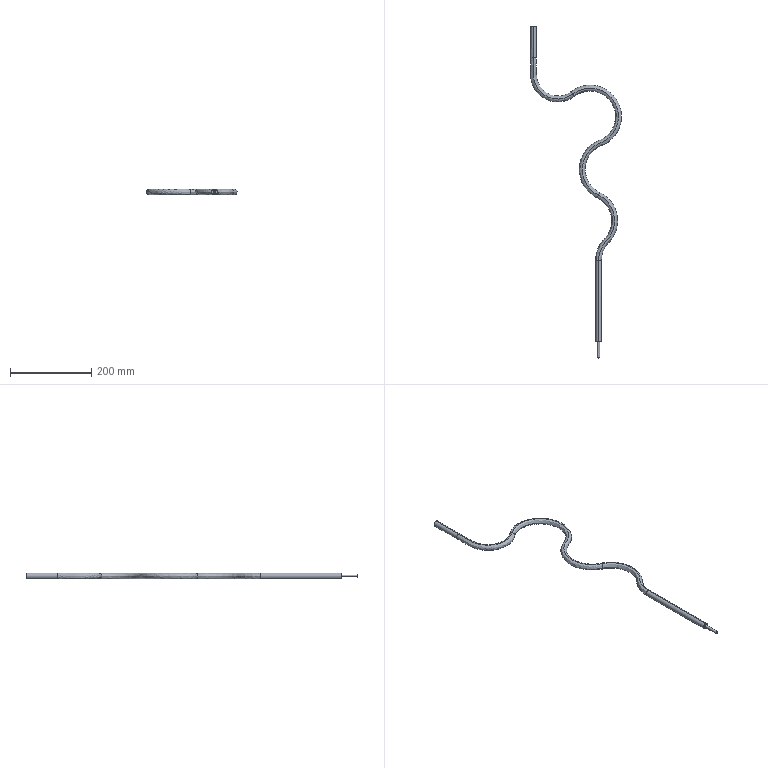Part | NX | features BREP 2 | 2 solids | 29 faces | box 223.745 x 818 x 14.512 mm | volume 140358 mm3 | cylinder 13 | spline 12 | plane 4 | commonest cylinder face diameters 6.35 x7 14.5 x4 3.91 x2